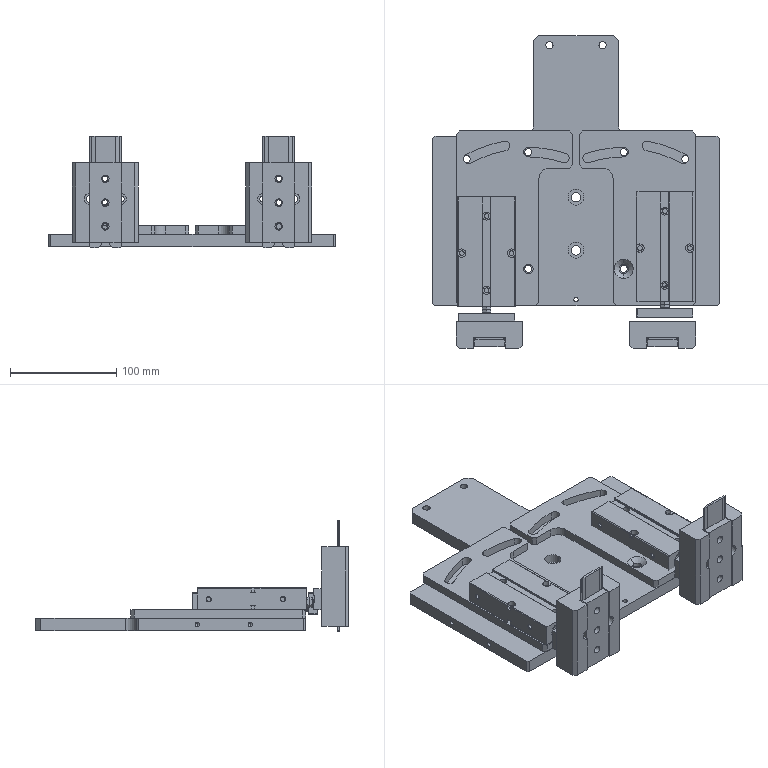Part | SolidWorks | features ReferencePattern 4, MirrorCompFeat 2 | 13 solids | 874 faces | box 270 x 295.093 x 105 mm | volume 1190493 mm3 | cylinder 414 | plane 344 | cone 116 | commonest cylinder face diameters 0.4 x60 1.52 x32 8 x32 9 x28 3.5 x24 16 x24